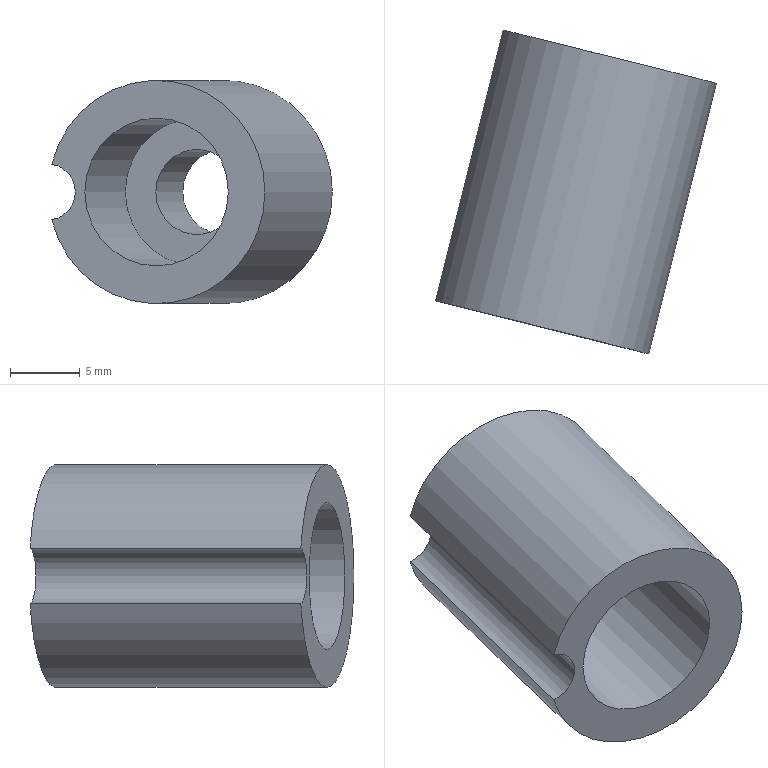Part | NX | features solid 2 | 1 solid | 7 faces | box 20.121 x 23.216 x 16 mm | volume 2609 mm3 | cylinder 4 | plane 3 | commonest cylinder face diameters 4 x1 6.1 x1 10.6 x1 16 x1
STEP:
#1=CARTESIAN_POINT('',(-953.368,239.924,104.711));
#2=VERTEX_POINT('',#1);
#3=CARTESIAN_POINT('',(-948.53,259.33,104.711));
#4=VERTEX_POINT('',#3);
#5=CARTESIAN_POINT('',(-950.949,249.627,104.711));
#6=DIRECTION('',(0.2419,0.9703,0.));
#7=VECTOR('',#6,1000.);
#8=LINE('',#5,#7);
#9=EDGE_CURVE('',#2,#4,#8,.T.);
#10=ORIENTED_EDGE('',*,*,#9,.F.);
#11=CARTESIAN_POINT('',(-953.368,239.924,100.743));
#12=VERTEX_POINT('',#11);
#13=CARTESIAN_POINT('',(-945.848,238.049,102.727));
#14=DIRECTION('',(0.2419,0.9703,0.));
#15=DIRECTION('',(-0.9703,0.2419,0.));
#16=AXIS2_PLACEMENT_3D('',#13,#14,#15);
#17=CIRCLE('',#16,8.);
#18=EDGE_CURVE('',#2,#12,#17,.T.);
#19=ORIENTED_EDGE('',*,*,#18,.T.);
#20=CARTESIAN_POINT('',(-948.53,259.33,100.743));
#21=VERTEX_POINT('',#20);
#22=CARTESIAN_POINT('',(-950.949,249.627,100.743));
#23=DIRECTION('',(0.2419,0.9703,0.));
#24=VECTOR('',#23,1000.);
#25=LINE('',#22,#24);
#26=EDGE_CURVE('',#21,#12,#25,.F.);
#27=ORIENTED_EDGE('',*,*,#26,.F.);
#28=CARTESIAN_POINT('',(-941.01,257.455,102.727));
#29=DIRECTION('',(0.2419,0.9703,0.));
#30=DIRECTION('',(-0.9703,0.2419,0.));
#31=AXIS2_PLACEMENT_3D('',#28,#29,#30);
#32=CIRCLE('',#31,8.);
#33=EDGE_CURVE('',#4,#21,#32,.T.);
#34=ORIENTED_EDGE('',*,*,#33,.F.);
#35=EDGE_LOOP('',(#10,#19,#27,#34));
#36=FACE_BOUND('',#35,.T.);
#37=CARTESIAN_POINT('',(-945.848,238.049,102.727));
#38=DIRECTION('',(0.2419,0.9703,0.));
#39=DIRECTION('',(-0.9703,0.2419,0.));
#40=AXIS2_PLACEMENT_3D('',#37,#38,#39);
#41=CYLINDRICAL_SURFACE('',#40,8.);
#42=ADVANCED_FACE('',(#36),#41,.T.);
#43=CARTESIAN_POINT('',(-950.991,239.331,102.727));
#44=VERTEX_POINT('',#43);
#45=CARTESIAN_POINT('',(-945.848,238.049,102.727));
#46=DIRECTION('',(0.2419,0.9703,0.));
#47=DIRECTION('',(-0.9703,0.2419,0.));
#48=AXIS2_PLACEMENT_3D('',#45,#46,#47);
#49=CIRCLE('',#48,5.3);
#50=EDGE_CURVE('',#44,#44,#49,.T.);
#51=ORIENTED_EDGE('',*,*,#50,.T.);
#52=EDGE_LOOP('',(#51));
#53=FACE_BOUND('',#52,.T.);
#54=ORIENTED_EDGE('',*,*,#18,.F.);
#55=CARTESIAN_POINT('',(-953.611,239.984,102.727));
#56=DIRECTION('',(0.2419,0.9703,0.));
#57=DIRECTION('',(-0.9703,0.2419,0.));
#58=AXIS2_PLACEMENT_3D('',#55,#56,#57);
#59=CIRCLE('',#58,2.);
#60=EDGE_CURVE('',#2,#12,#59,.T.);
#61=ORIENTED_EDGE('',*,*,#60,.T.);
#62=EDGE_LOOP('',(#54,#61));
#63=FACE_BOUND('',#62,.T.);
#64=CARTESIAN_POINT('',(-945.848,238.049,102.727));
#65=DIRECTION('',(0.2419,0.9703,0.));
#66=DIRECTION('',(-0.9703,0.2419,0.));
#67=AXIS2_PLACEMENT_3D('',#64,#65,#66);
#68=PLANE('',#67);
#69=ADVANCED_FACE('',(#53,#63),#68,.F.);
#70=CARTESIAN_POINT('',(-943.969,258.193,102.727));
#71=VERTEX_POINT('',#70);
#72=CARTESIAN_POINT('',(-941.01,257.455,102.727));
#73=DIRECTION('',(0.2419,0.9703,0.));
#74=DIRECTION('',(-0.9703,0.2419,0.));
#75=AXIS2_PLACEMENT_3D('',#72,#73,#74);
#76=CIRCLE('',#75,3.05);
#77=EDGE_CURVE('',#71,#71,#76,.T.);
#78=ORIENTED_EDGE('',*,*,#77,.F.);
#79=EDGE_LOOP('',(#78));
#80=FACE_BOUND('',#79,.T.);
#81=CARTESIAN_POINT('',(-948.772,259.39,102.727));
#82=DIRECTION('',(0.2419,0.9703,0.));
#83=DIRECTION('',(-0.9703,0.2419,0.));
#84=AXIS2_PLACEMENT_3D('',#81,#82,#83);
#85=CIRCLE('',#84,2.);
#86=EDGE_CURVE('',#4,#21,#85,.T.);
#87=ORIENTED_EDGE('',*,*,#86,.F.);
#88=ORIENTED_EDGE('',*,*,#33,.T.);
#89=EDGE_LOOP('',(#87,#88));
#90=FACE_BOUND('',#89,.T.);
#91=CARTESIAN_POINT('',(-941.01,257.455,102.727));
#92=DIRECTION('',(0.2419,0.9703,0.));
#93=DIRECTION('',(-0.9703,0.2419,0.));
#94=AXIS2_PLACEMENT_3D('',#91,#92,#93);
#95=PLANE('',#94);
#96=ADVANCED_FACE('',(#80,#90),#95,.T.);
#97=ORIENTED_EDGE('',*,*,#50,.F.);
#98=EDGE_LOOP('',(#97));
#99=FACE_BOUND('',#98,.T.);
#100=CARTESIAN_POINT('',(-948.088,250.975,102.727));
#101=VERTEX_POINT('',#100);
#102=CARTESIAN_POINT('',(-942.945,249.692,102.727));
#103=DIRECTION('',(0.2419,0.9703,0.));
#104=DIRECTION('',(-0.9703,0.2419,0.));
#105=AXIS2_PLACEMENT_3D('',#102,#103,#104);
#106=CIRCLE('',#105,5.3);
#107=EDGE_CURVE('',#101,#101,#106,.T.);
#108=ORIENTED_EDGE('',*,*,#107,.T.);
#109=EDGE_LOOP('',(#108));
#110=FACE_BOUND('',#109,.T.);
#111=CARTESIAN_POINT('',(-945.848,238.049,102.727));
#112=DIRECTION('',(0.2419,0.9703,0.));
#113=DIRECTION('',(-0.9703,0.2419,0.));
#114=AXIS2_PLACEMENT_3D('',#111,#112,#113);
#115=CYLINDRICAL_SURFACE('',#114,5.3);
#116=ADVANCED_FACE('',(#99,#110),#115,.F.);
#117=CARTESIAN_POINT('',(-945.905,250.43,102.727));
#118=VERTEX_POINT('',#117);
#119=CARTESIAN_POINT('',(-942.945,249.692,102.727));
#120=DIRECTION('',(0.2419,0.9703,0.));
#121=DIRECTION('',(-0.9703,0.2419,0.));
#122=AXIS2_PLACEMENT_3D('',#119,#120,#121);
#123=CIRCLE('',#122,3.05);
#124=EDGE_CURVE('',#118,#118,#123,.T.);
#125=ORIENTED_EDGE('',*,*,#124,.T.);
#126=EDGE_LOOP('',(#125));
#127=FACE_BOUND('',#126,.T.);
#128=ORIENTED_EDGE('',*,*,#107,.F.);
#129=EDGE_LOOP('',(#128));
#130=FACE_BOUND('',#129,.T.);
#131=CARTESIAN_POINT('',(-942.945,249.692,102.727));
#132=DIRECTION('',(0.2419,0.9703,0.));
#133=DIRECTION('',(-0.9703,0.2419,0.));
#134=AXIS2_PLACEMENT_3D('',#131,#132,#133);
#135=PLANE('',#134);
#136=ADVANCED_FACE('',(#127,#130),#135,.F.);
#137=ORIENTED_EDGE('',*,*,#9,.T.);
#138=ORIENTED_EDGE('',*,*,#86,.T.);
#139=ORIENTED_EDGE('',*,*,#26,.T.);
#140=ORIENTED_EDGE('',*,*,#60,.F.);
#141=EDGE_LOOP('',(#137,#138,#139,#140));
#142=FACE_BOUND('',#141,.T.);
#143=CARTESIAN_POINT('',(-953.611,239.984,102.727));
#144=DIRECTION('',(0.2419,0.9703,0.));
#145=DIRECTION('',(-0.9703,0.2419,0.));
#146=AXIS2_PLACEMENT_3D('',#143,#144,#145);
#147=CYLINDRICAL_SURFACE('',#146,2.);
#148=ADVANCED_FACE('',(#142),#147,.F.);
#149=ORIENTED_EDGE('',*,*,#77,.T.);
#150=EDGE_LOOP('',(#149));
#151=FACE_BOUND('',#150,.T.);
#152=ORIENTED_EDGE('',*,*,#124,.F.);
#153=EDGE_LOOP('',(#152));
#154=FACE_BOUND('',#153,.T.);
#155=CARTESIAN_POINT('',(-945.848,238.049,102.727));
#156=DIRECTION('',(0.2419,0.9703,0.));
#157=DIRECTION('',(-0.9703,0.2419,0.));
#158=AXIS2_PLACEMENT_3D('',#155,#156,#157);
#159=CYLINDRICAL_SURFACE('',#158,3.05);
#160=ADVANCED_FACE('',(#151,#154),#159,.F.);
#161=CLOSED_SHELL('',(#42,#69,#96,#116,#136,#148,#160));
#162=MANIFOLD_SOLID_BREP('',#161);
#163=(LENGTH_UNIT()NAMED_UNIT(*)SI_UNIT(.MILLI.,.METRE.));
#164=UNCERTAINTY_MEASURE_WITH_UNIT(LENGTH_MEASURE(0.00001),#163,'','');
#165=(NAMED_UNIT(*)PLANE_ANGLE_UNIT()SI_UNIT($,.RADIAN.));
#166=(NAMED_UNIT(*)SI_UNIT($,.STERADIAN.)SOLID_ANGLE_UNIT());
#167=(GEOMETRIC_REPRESENTATION_CONTEXT(3)GLOBAL_UNCERTAINTY_ASSIGNED_CONTEXT((#164))GLOBAL_UNIT_ASSIGNED_CONTEXT((#163,#165,#166))REPRESENTATION_CONTEXT('',''));
#168=ADVANCED_BREP_SHAPE_REPRESENTATION('',(#162),#167);